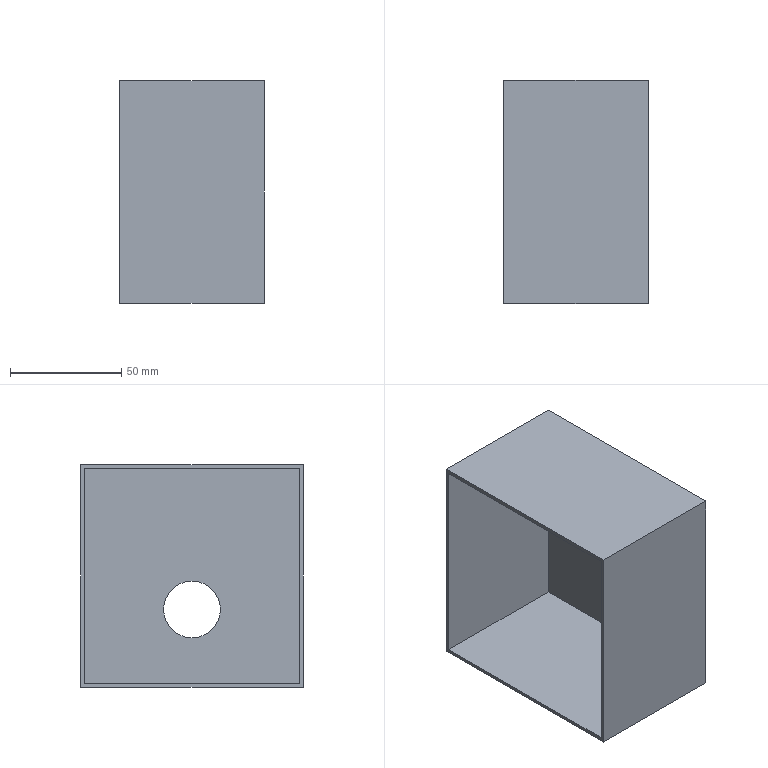Part | NX | features solid 2 | 1 solid | 12 faces | box 65 x 100 x 100 mm | volume 55110 mm3 | plane 11 | cylinder 1 | commonest cylinder face diameters 25.5 x1
STEP:
#1=CARTESIAN_POINT('',(-1085.,-220.,-570.));
#2=VERTEX_POINT('',#1);
#3=CARTESIAN_POINT('',(-1085.,-320.,-570.));
#4=VERTEX_POINT('',#3);
#5=CARTESIAN_POINT('',(-1085.,-210.,-570.));
#6=DIRECTION('',(0.,-1.,0.));
#7=VECTOR('',#6,1000.);
#8=LINE('',#5,#7);
#9=EDGE_CURVE('',#2,#4,#8,.T.);
#10=ORIENTED_EDGE('',*,*,#9,.F.);
#11=CARTESIAN_POINT('',(-1020.,-220.,-570.));
#12=VERTEX_POINT('',#11);
#13=CARTESIAN_POINT('',(-1015.,-220.,-570.));
#14=DIRECTION('',(-1.,0.,0.));
#15=VECTOR('',#14,1000.);
#16=LINE('',#13,#15);
#17=EDGE_CURVE('',#12,#2,#16,.T.);
#18=ORIENTED_EDGE('',*,*,#17,.F.);
#19=CARTESIAN_POINT('',(-1020.,-320.,-570.));
#20=VERTEX_POINT('',#19);
#21=CARTESIAN_POINT('',(-1020.,-210.,-570.));
#22=DIRECTION('',(0.,-1.,0.));
#23=VECTOR('',#22,1000.);
#24=LINE('',#21,#23);
#25=EDGE_CURVE('',#12,#20,#24,.T.);
#26=ORIENTED_EDGE('',*,*,#25,.T.);
#27=CARTESIAN_POINT('',(-1015.,-320.,-570.));
#28=DIRECTION('',(-1.,0.,0.));
#29=VECTOR('',#28,1000.);
#30=LINE('',#27,#29);
#31=EDGE_CURVE('',#20,#4,#30,.T.);
#32=ORIENTED_EDGE('',*,*,#31,.T.);
#33=EDGE_LOOP('',(#10,#18,#26,#32));
#34=FACE_BOUND('',#33,.T.);
#35=CARTESIAN_POINT('',(-1015.,-210.,-570.));
#36=DIRECTION('',(0.,0.,1.));
#37=DIRECTION('',(-1.,0.,0.));
#38=AXIS2_PLACEMENT_3D('',#35,#36,#37);
#39=PLANE('',#38);
#40=ADVANCED_FACE('',(#34),#39,.F.);
#41=CARTESIAN_POINT('',(-1085.,-220.,-470.));
#42=VERTEX_POINT('',#41);
#43=CARTESIAN_POINT('',(-1085.,-220.,-580.));
#44=DIRECTION('',(0.,0.,1.));
#45=VECTOR('',#44,1000.);
#46=LINE('',#43,#45);
#47=EDGE_CURVE('',#2,#42,#46,.T.);
#48=ORIENTED_EDGE('',*,*,#47,.T.);
#49=CARTESIAN_POINT('',(-1020.,-220.,-470.));
#50=VERTEX_POINT('',#49);
#51=CARTESIAN_POINT('',(-1015.,-220.,-470.));
#52=DIRECTION('',(-1.,0.,0.));
#53=VECTOR('',#52,1000.);
#54=LINE('',#51,#53);
#55=EDGE_CURVE('',#50,#42,#54,.T.);
#56=ORIENTED_EDGE('',*,*,#55,.F.);
#57=CARTESIAN_POINT('',(-1020.,-220.,-580.));
#58=DIRECTION('',(0.,0.,1.));
#59=VECTOR('',#58,1000.);
#60=LINE('',#57,#59);
#61=EDGE_CURVE('',#12,#50,#60,.T.);
#62=ORIENTED_EDGE('',*,*,#61,.F.);
#63=ORIENTED_EDGE('',*,*,#17,.T.);
#64=EDGE_LOOP('',(#48,#56,#62,#63));
#65=FACE_BOUND('',#64,.T.);
#66=CARTESIAN_POINT('',(-1015.,-220.,-580.));
#67=DIRECTION('',(0.,1.,0.));
#68=DIRECTION('',(0.,0.,1.));
#69=AXIS2_PLACEMENT_3D('',#66,#67,#68);
#70=PLANE('',#69);
#71=ADVANCED_FACE('',(#65),#70,.T.);
#72=CARTESIAN_POINT('',(-1085.,-320.,-470.));
#73=VERTEX_POINT('',#72);
#74=CARTESIAN_POINT('',(-1085.,-210.,-470.));
#75=DIRECTION('',(0.,-1.,0.));
#76=VECTOR('',#75,1000.);
#77=LINE('',#74,#76);
#78=EDGE_CURVE('',#42,#73,#77,.T.);
#79=ORIENTED_EDGE('',*,*,#78,.T.);
#80=CARTESIAN_POINT('',(-1020.,-320.,-470.));
#81=VERTEX_POINT('',#80);
#82=CARTESIAN_POINT('',(-1015.,-320.,-470.));
#83=DIRECTION('',(-1.,0.,0.));
#84=VECTOR('',#83,1000.);
#85=LINE('',#82,#84);
#86=EDGE_CURVE('',#81,#73,#85,.T.);
#87=ORIENTED_EDGE('',*,*,#86,.F.);
#88=CARTESIAN_POINT('',(-1020.,-210.,-470.));
#89=DIRECTION('',(0.,-1.,0.));
#90=VECTOR('',#89,1000.);
#91=LINE('',#88,#90);
#92=EDGE_CURVE('',#50,#81,#91,.T.);
#93=ORIENTED_EDGE('',*,*,#92,.F.);
#94=ORIENTED_EDGE('',*,*,#55,.T.);
#95=EDGE_LOOP('',(#79,#87,#93,#94));
#96=FACE_BOUND('',#95,.T.);
#97=CARTESIAN_POINT('',(-1015.,-210.,-470.));
#98=DIRECTION('',(0.,0.,1.));
#99=DIRECTION('',(-1.,0.,0.));
#100=AXIS2_PLACEMENT_3D('',#97,#98,#99);
#101=PLANE('',#100);
#102=ADVANCED_FACE('',(#96),#101,.T.);
#103=CARTESIAN_POINT('',(-1085.,-320.,-580.));
#104=DIRECTION('',(0.,0.,1.));
#105=VECTOR('',#104,1000.);
#106=LINE('',#103,#105);
#107=EDGE_CURVE('',#4,#73,#106,.T.);
#108=ORIENTED_EDGE('',*,*,#107,.F.);
#109=ORIENTED_EDGE('',*,*,#31,.F.);
#110=CARTESIAN_POINT('',(-1020.,-320.,-580.));
#111=DIRECTION('',(0.,0.,1.));
#112=VECTOR('',#111,1000.);
#113=LINE('',#110,#112);
#114=EDGE_CURVE('',#20,#81,#113,.T.);
#115=ORIENTED_EDGE('',*,*,#114,.T.);
#116=ORIENTED_EDGE('',*,*,#86,.T.);
#117=EDGE_LOOP('',(#108,#109,#115,#116));
#118=FACE_BOUND('',#117,.T.);
#119=CARTESIAN_POINT('',(-1015.,-320.,-580.));
#120=DIRECTION('',(0.,1.,0.));
#121=DIRECTION('',(0.,0.,1.));
#122=AXIS2_PLACEMENT_3D('',#119,#120,#121);
#123=PLANE('',#122);
#124=ADVANCED_FACE('',(#118),#123,.F.);
#125=CARTESIAN_POINT('',(-1020.,-270.,-522.25));
#126=VERTEX_POINT('',#125);
#127=CARTESIAN_POINT('',(-1020.,-270.,-535.));
#128=DIRECTION('',(-1.,0.,0.));
#129=DIRECTION('',(0.,0.,1.));
#130=AXIS2_PLACEMENT_3D('',#127,#128,#129);
#131=CIRCLE('',#130,12.75);
#132=EDGE_CURVE('',#126,#126,#131,.T.);
#133=ORIENTED_EDGE('',*,*,#132,.T.);
#134=EDGE_LOOP('',(#133));
#135=FACE_BOUND('',#134,.T.);
#136=ORIENTED_EDGE('',*,*,#25,.F.);
#137=ORIENTED_EDGE('',*,*,#61,.T.);
#138=ORIENTED_EDGE('',*,*,#92,.T.);
#139=ORIENTED_EDGE('',*,*,#114,.F.);
#140=EDGE_LOOP('',(#136,#137,#138,#139));
#141=FACE_BOUND('',#140,.T.);
#142=CARTESIAN_POINT('',(-1020.,-210.,-580.));
#143=DIRECTION('',(-1.,0.,0.));
#144=DIRECTION('',(0.,0.,-1.));
#145=AXIS2_PLACEMENT_3D('',#142,#143,#144);
#146=PLANE('',#145);
#147=ADVANCED_FACE('',(#135,#141),#146,.F.);
#148=CARTESIAN_POINT('',(-1085.,-221.6,-568.4));
#149=VERTEX_POINT('',#148);
#150=CARTESIAN_POINT('',(-1085.,-318.4,-568.4));
#151=VERTEX_POINT('',#150);
#152=CARTESIAN_POINT('',(-1085.,-210.,-568.4));
#153=DIRECTION('',(0.,-1.,0.));
#154=VECTOR('',#153,1000.);
#155=LINE('',#152,#154);
#156=EDGE_CURVE('',#149,#151,#155,.T.);
#157=ORIENTED_EDGE('',*,*,#156,.F.);
#158=CARTESIAN_POINT('',(-1085.,-221.6,-471.6));
#159=VERTEX_POINT('',#158);
#160=CARTESIAN_POINT('',(-1085.,-221.6,-580.));
#161=DIRECTION('',(0.,0.,1.));
#162=VECTOR('',#161,1000.);
#163=LINE('',#160,#162);
#164=EDGE_CURVE('',#149,#159,#163,.T.);
#165=ORIENTED_EDGE('',*,*,#164,.T.);
#166=CARTESIAN_POINT('',(-1085.,-318.4,-471.6));
#167=VERTEX_POINT('',#166);
#168=CARTESIAN_POINT('',(-1085.,-210.,-471.6));
#169=DIRECTION('',(0.,-1.,0.));
#170=VECTOR('',#169,1000.);
#171=LINE('',#168,#170);
#172=EDGE_CURVE('',#159,#167,#171,.T.);
#173=ORIENTED_EDGE('',*,*,#172,.T.);
#174=CARTESIAN_POINT('',(-1085.,-318.4,-580.));
#175=DIRECTION('',(0.,0.,1.));
#176=VECTOR('',#175,1000.);
#177=LINE('',#174,#176);
#178=EDGE_CURVE('',#151,#167,#177,.T.);
#179=ORIENTED_EDGE('',*,*,#178,.F.);
#180=EDGE_LOOP('',(#157,#165,#173,#179));
#181=FACE_BOUND('',#180,.T.);
#182=ORIENTED_EDGE('',*,*,#9,.T.);
#183=ORIENTED_EDGE('',*,*,#107,.T.);
#184=ORIENTED_EDGE('',*,*,#78,.F.);
#185=ORIENTED_EDGE('',*,*,#47,.F.);
#186=EDGE_LOOP('',(#182,#183,#184,#185));
#187=FACE_BOUND('',#186,.T.);
#188=CARTESIAN_POINT('',(-1085.,-210.,-580.));
#189=DIRECTION('',(-1.,0.,0.));
#190=DIRECTION('',(0.,0.,-1.));
#191=AXIS2_PLACEMENT_3D('',#188,#189,#190);
#192=PLANE('',#191);
#193=ADVANCED_FACE('',(#181,#187),#192,.T.);
#194=ORIENTED_EDGE('',*,*,#156,.T.);
#195=CARTESIAN_POINT('',(-1021.6,-318.4,-568.4));
#196=VERTEX_POINT('',#195);
#197=CARTESIAN_POINT('',(-1015.,-318.4,-568.4));
#198=DIRECTION('',(-1.,0.,0.));
#199=VECTOR('',#198,1000.);
#200=LINE('',#197,#199);
#201=EDGE_CURVE('',#196,#151,#200,.T.);
#202=ORIENTED_EDGE('',*,*,#201,.F.);
#203=CARTESIAN_POINT('',(-1021.6,-221.6,-568.4));
#204=VERTEX_POINT('',#203);
#205=CARTESIAN_POINT('',(-1021.6,-210.,-568.4));
#206=DIRECTION('',(0.,-1.,0.));
#207=VECTOR('',#206,1000.);
#208=LINE('',#205,#207);
#209=EDGE_CURVE('',#204,#196,#208,.T.);
#210=ORIENTED_EDGE('',*,*,#209,.F.);
#211=CARTESIAN_POINT('',(-1015.,-221.6,-568.4));
#212=DIRECTION('',(-1.,0.,0.));
#213=VECTOR('',#212,1000.);
#214=LINE('',#211,#213);
#215=EDGE_CURVE('',#204,#149,#214,.T.);
#216=ORIENTED_EDGE('',*,*,#215,.T.);
#217=EDGE_LOOP('',(#194,#202,#210,#216));
#218=FACE_BOUND('',#217,.T.);
#219=CARTESIAN_POINT('',(-1015.,-210.,-568.4));
#220=DIRECTION('',(0.,0.,1.));
#221=DIRECTION('',(-1.,0.,0.));
#222=AXIS2_PLACEMENT_3D('',#219,#220,#221);
#223=PLANE('',#222);
#224=ADVANCED_FACE('',(#218),#223,.T.);
#225=ORIENTED_EDGE('',*,*,#164,.F.);
#226=ORIENTED_EDGE('',*,*,#215,.F.);
#227=CARTESIAN_POINT('',(-1021.6,-221.6,-471.6));
#228=VERTEX_POINT('',#227);
#229=CARTESIAN_POINT('',(-1021.6,-221.6,-580.));
#230=DIRECTION('',(0.,0.,1.));
#231=VECTOR('',#230,1000.);
#232=LINE('',#229,#231);
#233=EDGE_CURVE('',#204,#228,#232,.T.);
#234=ORIENTED_EDGE('',*,*,#233,.T.);
#235=CARTESIAN_POINT('',(-1015.,-221.6,-471.6));
#236=DIRECTION('',(-1.,0.,0.));
#237=VECTOR('',#236,1000.);
#238=LINE('',#235,#237);
#239=EDGE_CURVE('',#228,#159,#238,.T.);
#240=ORIENTED_EDGE('',*,*,#239,.T.);
#241=EDGE_LOOP('',(#225,#226,#234,#240));
#242=FACE_BOUND('',#241,.T.);
#243=CARTESIAN_POINT('',(-1015.,-221.6,-580.));
#244=DIRECTION('',(0.,1.,0.));
#245=DIRECTION('',(0.,0.,1.));
#246=AXIS2_PLACEMENT_3D('',#243,#244,#245);
#247=PLANE('',#246);
#248=ADVANCED_FACE('',(#242),#247,.F.);
#249=ORIENTED_EDGE('',*,*,#172,.F.);
#250=ORIENTED_EDGE('',*,*,#239,.F.);
#251=CARTESIAN_POINT('',(-1021.6,-318.4,-471.6));
#252=VERTEX_POINT('',#251);
#253=CARTESIAN_POINT('',(-1021.6,-210.,-471.6));
#254=DIRECTION('',(0.,-1.,0.));
#255=VECTOR('',#254,1000.);
#256=LINE('',#253,#255);
#257=EDGE_CURVE('',#228,#252,#256,.T.);
#258=ORIENTED_EDGE('',*,*,#257,.T.);
#259=CARTESIAN_POINT('',(-1015.,-318.4,-471.6));
#260=DIRECTION('',(-1.,0.,0.));
#261=VECTOR('',#260,1000.);
#262=LINE('',#259,#261);
#263=EDGE_CURVE('',#252,#167,#262,.T.);
#264=ORIENTED_EDGE('',*,*,#263,.T.);
#265=EDGE_LOOP('',(#249,#250,#258,#264));
#266=FACE_BOUND('',#265,.T.);
#267=CARTESIAN_POINT('',(-1015.,-210.,-471.6));
#268=DIRECTION('',(0.,0.,1.));
#269=DIRECTION('',(-1.,0.,0.));
#270=AXIS2_PLACEMENT_3D('',#267,#268,#269);
#271=PLANE('',#270);
#272=ADVANCED_FACE('',(#266),#271,.F.);
#273=ORIENTED_EDGE('',*,*,#178,.T.);
#274=ORIENTED_EDGE('',*,*,#263,.F.);
#275=CARTESIAN_POINT('',(-1021.6,-318.4,-580.));
#276=DIRECTION('',(0.,0.,1.));
#277=VECTOR('',#276,1000.);
#278=LINE('',#275,#277);
#279=EDGE_CURVE('',#196,#252,#278,.T.);
#280=ORIENTED_EDGE('',*,*,#279,.F.);
#281=ORIENTED_EDGE('',*,*,#201,.T.);
#282=EDGE_LOOP('',(#273,#274,#280,#281));
#283=FACE_BOUND('',#282,.T.);
#284=CARTESIAN_POINT('',(-1015.,-318.4,-580.));
#285=DIRECTION('',(0.,1.,0.));
#286=DIRECTION('',(0.,0.,1.));
#287=AXIS2_PLACEMENT_3D('',#284,#285,#286);
#288=PLANE('',#287);
#289=ADVANCED_FACE('',(#283),#288,.T.);
#290=CARTESIAN_POINT('',(-1021.6,-270.,-547.75));
#291=VERTEX_POINT('',#290);
#292=CARTESIAN_POINT('',(-1021.6,-270.,-535.));
#293=DIRECTION('',(1.,0.,0.));
#294=DIRECTION('',(0.,0.,-1.));
#295=AXIS2_PLACEMENT_3D('',#292,#293,#294);
#296=CIRCLE('',#295,12.75);
#297=EDGE_CURVE('',#291,#291,#296,.T.);
#298=ORIENTED_EDGE('',*,*,#297,.T.);
#299=EDGE_LOOP('',(#298));
#300=FACE_BOUND('',#299,.T.);
#301=ORIENTED_EDGE('',*,*,#209,.T.);
#302=ORIENTED_EDGE('',*,*,#279,.T.);
#303=ORIENTED_EDGE('',*,*,#257,.F.);
#304=ORIENTED_EDGE('',*,*,#233,.F.);
#305=EDGE_LOOP('',(#301,#302,#303,#304));
#306=FACE_BOUND('',#305,.T.);
#307=CARTESIAN_POINT('',(-1021.6,-210.,-580.));
#308=DIRECTION('',(-1.,0.,0.));
#309=DIRECTION('',(0.,0.,-1.));
#310=AXIS2_PLACEMENT_3D('',#307,#308,#309);
#311=PLANE('',#310);
#312=ADVANCED_FACE('',(#300,#306),#311,.T.);
#313=ORIENTED_EDGE('',*,*,#297,.F.);
#314=EDGE_LOOP('',(#313));
#315=FACE_BOUND('',#314,.T.);
#316=ORIENTED_EDGE('',*,*,#132,.F.);
#317=EDGE_LOOP('',(#316));
#318=FACE_BOUND('',#317,.T.);
#319=CARTESIAN_POINT('',(-1021.6,-270.,-535.));
#320=DIRECTION('',(1.,0.,0.));
#321=DIRECTION('',(0.,0.,-1.));
#322=AXIS2_PLACEMENT_3D('',#319,#320,#321);
#323=CYLINDRICAL_SURFACE('',#322,12.75);
#324=ADVANCED_FACE('',(#315,#318),#323,.F.);
#325=CLOSED_SHELL('',(#40,#71,#102,#124,#147,#193,#224,#248,#272,#289,#312,#324));
#326=MANIFOLD_SOLID_BREP('',#325);
#327=(LENGTH_UNIT()NAMED_UNIT(*)SI_UNIT(.MILLI.,.METRE.));
#328=UNCERTAINTY_MEASURE_WITH_UNIT(LENGTH_MEASURE(0.00001),#327,'','');
#329=(NAMED_UNIT(*)PLANE_ANGLE_UNIT()SI_UNIT($,.RADIAN.));
#330=(NAMED_UNIT(*)SI_UNIT($,.STERADIAN.)SOLID_ANGLE_UNIT());
#331=(GEOMETRIC_REPRESENTATION_CONTEXT(3)GLOBAL_UNCERTAINTY_ASSIGNED_CONTEXT((#328))GLOBAL_UNIT_ASSIGNED_CONTEXT((#327,#329,#330))REPRESENTATION_CONTEXT('',''));
#332=ADVANCED_BREP_SHAPE_REPRESENTATION('',(#326),#331);